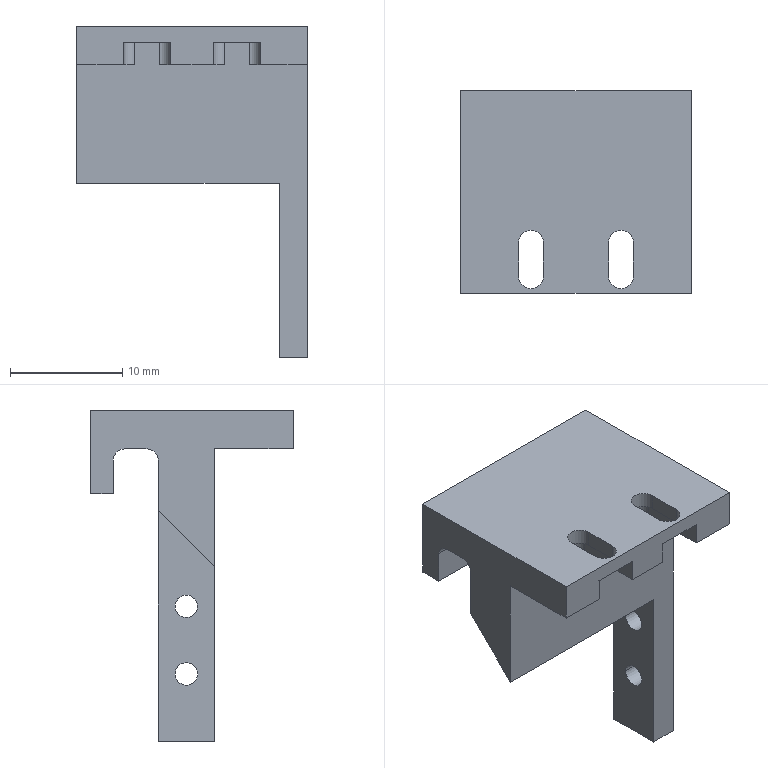Part | 1 solid | 42 faces | box 20.5 x 18 x 29.4 mm | volume 2312 mm3 | plane 26 | cylinder 16 | commonest cylinder face diameters 2 x10 2.2 x6
STEP:
#1=CARTESIAN_POINT('',(7.75,-0.5,-23.4));
#2=VERTEX_POINT('',#1);
#3=CARTESIAN_POINT('',(7.75,1.5,-23.4));
#4=VERTEX_POINT('',#3);
#5=CARTESIAN_POINT('',(7.75,0.5,-23.4));
#6=DIRECTION('',(-1.,0.,0.));
#7=DIRECTION('',(0.,1.,0.));
#8=AXIS2_PLACEMENT_3D('',#5,#6,#7);
#9=CIRCLE('',#8,1.);
#10=EDGE_CURVE('',#2,#4,#9,.T.);
#11=ORIENTED_EDGE('',*,*,#10,.T.);
#12=CARTESIAN_POINT('',(10.25,1.5,-23.4));
#13=VERTEX_POINT('',#12);
#14=CARTESIAN_POINT('',(10.25,1.5,-23.4));
#15=DIRECTION('',(1.,0.,0.));
#16=VECTOR('',#15,1000.);
#17=LINE('',#14,#16);
#18=EDGE_CURVE('',#13,#4,#17,.F.);
#19=ORIENTED_EDGE('',*,*,#18,.F.);
#20=CARTESIAN_POINT('',(10.25,-0.5,-23.4));
#21=VERTEX_POINT('',#20);
#22=CARTESIAN_POINT('',(10.25,0.5,-23.4));
#23=DIRECTION('',(1.,0.,0.));
#24=DIRECTION('',(0.,-1.,0.));
#25=AXIS2_PLACEMENT_3D('',#22,#23,#24);
#26=CIRCLE('',#25,1.);
#27=EDGE_CURVE('',#13,#21,#26,.T.);
#28=ORIENTED_EDGE('',*,*,#27,.T.);
#29=CARTESIAN_POINT('',(10.25,-0.5,-23.4));
#30=DIRECTION('',(1.,0.,0.));
#31=VECTOR('',#30,1000.);
#32=LINE('',#29,#31);
#33=EDGE_CURVE('',#21,#2,#32,.F.);
#34=ORIENTED_EDGE('',*,*,#33,.T.);
#35=EDGE_LOOP('',(#11,#19,#28,#34));
#36=FACE_BOUND('',#35,.T.);
#37=CARTESIAN_POINT('',(10.25,0.5,-23.4));
#38=DIRECTION('',(1.,0.,0.));
#39=DIRECTION('',(0.,1.,0.));
#40=AXIS2_PLACEMENT_3D('',#37,#38,#39);
#41=CYLINDRICAL_SURFACE('',#40,1.);
#42=ADVANCED_FACE('',(#36),#41,.F.);
#43=CARTESIAN_POINT('',(7.75,-0.5,-17.4));
#44=VERTEX_POINT('',#43);
#45=CARTESIAN_POINT('',(7.75,1.5,-17.4));
#46=VERTEX_POINT('',#45);
#47=CARTESIAN_POINT('',(7.75,0.5,-17.4));
#48=DIRECTION('',(-1.,0.,0.));
#49=DIRECTION('',(0.,1.,0.));
#50=AXIS2_PLACEMENT_3D('',#47,#48,#49);
#51=CIRCLE('',#50,1.);
#52=EDGE_CURVE('',#44,#46,#51,.T.);
#53=ORIENTED_EDGE('',*,*,#52,.T.);
#54=CARTESIAN_POINT('',(10.25,1.5,-17.4));
#55=VERTEX_POINT('',#54);
#56=CARTESIAN_POINT('',(10.25,1.5,-17.4));
#57=DIRECTION('',(1.,0.,0.));
#58=VECTOR('',#57,1000.);
#59=LINE('',#56,#58);
#60=EDGE_CURVE('',#55,#46,#59,.F.);
#61=ORIENTED_EDGE('',*,*,#60,.F.);
#62=CARTESIAN_POINT('',(10.25,-0.5,-17.4));
#63=VERTEX_POINT('',#62);
#64=CARTESIAN_POINT('',(10.25,0.5,-17.4));
#65=DIRECTION('',(1.,0.,0.));
#66=DIRECTION('',(0.,-1.,0.));
#67=AXIS2_PLACEMENT_3D('',#64,#65,#66);
#68=CIRCLE('',#67,1.);
#69=EDGE_CURVE('',#55,#63,#68,.T.);
#70=ORIENTED_EDGE('',*,*,#69,.T.);
#71=CARTESIAN_POINT('',(10.25,-0.5,-17.4));
#72=DIRECTION('',(1.,0.,0.));
#73=VECTOR('',#72,1000.);
#74=LINE('',#71,#73);
#75=EDGE_CURVE('',#63,#44,#74,.F.);
#76=ORIENTED_EDGE('',*,*,#75,.T.);
#77=EDGE_LOOP('',(#53,#61,#70,#76));
#78=FACE_BOUND('',#77,.T.);
#79=CARTESIAN_POINT('',(10.25,0.5,-17.4));
#80=DIRECTION('',(1.,0.,0.));
#81=DIRECTION('',(0.,1.,0.));
#82=AXIS2_PLACEMENT_3D('',#79,#80,#81);
#83=CYLINDRICAL_SURFACE('',#82,1.);
#84=ADVANCED_FACE('',(#78),#83,.F.);
#85=CARTESIAN_POINT('',(-4.,-8.6,0.));
#86=VERTEX_POINT('',#85);
#87=CARTESIAN_POINT('',(-5.1,-7.5,0.));
#88=VERTEX_POINT('',#87);
#89=CARTESIAN_POINT('',(-4.,-7.5,0.));
#90=DIRECTION('',(0.,0.,-1.));
#91=DIRECTION('',(0.,1.,0.));
#92=AXIS2_PLACEMENT_3D('',#89,#90,#91);
#93=CIRCLE('',#92,1.1);
#94=EDGE_CURVE('',#86,#88,#93,.T.);
#95=ORIENTED_EDGE('',*,*,#94,.F.);
#96=CARTESIAN_POINT('',(-4.,-8.6,-1.4));
#97=VERTEX_POINT('',#96);
#98=CARTESIAN_POINT('',(-4.,-8.6,0.));
#99=DIRECTION('',(0.,0.,-1.));
#100=VECTOR('',#99,1000.);
#101=LINE('',#98,#100);
#102=EDGE_CURVE('',#86,#97,#101,.T.);
#103=ORIENTED_EDGE('',*,*,#102,.T.);
#104=CARTESIAN_POINT('',(-5.1,-7.5,-1.4));
#105=VERTEX_POINT('',#104);
#106=CARTESIAN_POINT('',(-4.,-7.5,-1.4));
#107=DIRECTION('',(0.,0.,-1.));
#108=DIRECTION('',(0.,1.,0.));
#109=AXIS2_PLACEMENT_3D('',#106,#107,#108);
#110=CIRCLE('',#109,1.1);
#111=EDGE_CURVE('',#97,#105,#110,.T.);
#112=ORIENTED_EDGE('',*,*,#111,.T.);
#113=CARTESIAN_POINT('',(-5.1,-7.5,0.));
#114=DIRECTION('',(0.,0.,-1.));
#115=VECTOR('',#114,1000.);
#116=LINE('',#113,#115);
#117=EDGE_CURVE('',#88,#105,#116,.T.);
#118=ORIENTED_EDGE('',*,*,#117,.F.);
#119=EDGE_LOOP('',(#95,#103,#112,#118));
#120=FACE_BOUND('',#119,.T.);
#121=CARTESIAN_POINT('',(-4.,-7.5,0.));
#122=DIRECTION('',(0.,0.,-1.));
#123=DIRECTION('',(0.,1.,0.));
#124=AXIS2_PLACEMENT_3D('',#121,#122,#123);
#125=CYLINDRICAL_SURFACE('',#124,1.1);
#126=ADVANCED_FACE('',(#120),#125,.F.);
#127=CARTESIAN_POINT('',(4.,-8.6,0.));
#128=VERTEX_POINT('',#127);
#129=CARTESIAN_POINT('',(2.9,-7.5,0.));
#130=VERTEX_POINT('',#129);
#131=CARTESIAN_POINT('',(4.,-7.5,0.));
#132=DIRECTION('',(0.,0.,-1.));
#133=DIRECTION('',(0.,-1.,0.));
#134=AXIS2_PLACEMENT_3D('',#131,#132,#133);
#135=CIRCLE('',#134,1.1);
#136=EDGE_CURVE('',#128,#130,#135,.T.);
#137=ORIENTED_EDGE('',*,*,#136,.F.);
#138=CARTESIAN_POINT('',(4.,-8.6,-1.4));
#139=VERTEX_POINT('',#138);
#140=CARTESIAN_POINT('',(4.,-8.6,0.));
#141=DIRECTION('',(0.,0.,-1.));
#142=VECTOR('',#141,1000.);
#143=LINE('',#140,#142);
#144=EDGE_CURVE('',#128,#139,#143,.T.);
#145=ORIENTED_EDGE('',*,*,#144,.T.);
#146=CARTESIAN_POINT('',(2.9,-7.5,-1.4));
#147=VERTEX_POINT('',#146);
#148=CARTESIAN_POINT('',(4.,-7.5,-1.4));
#149=DIRECTION('',(0.,0.,1.));
#150=DIRECTION('',(0.,-1.,0.));
#151=AXIS2_PLACEMENT_3D('',#148,#149,#150);
#152=CIRCLE('',#151,1.1);
#153=EDGE_CURVE('',#147,#139,#152,.T.);
#154=ORIENTED_EDGE('',*,*,#153,.F.);
#155=CARTESIAN_POINT('',(2.9,-7.5,0.));
#156=DIRECTION('',(0.,0.,-1.));
#157=VECTOR('',#156,1000.);
#158=LINE('',#155,#157);
#159=EDGE_CURVE('',#130,#147,#158,.T.);
#160=ORIENTED_EDGE('',*,*,#159,.F.);
#161=EDGE_LOOP('',(#137,#145,#154,#160));
#162=FACE_BOUND('',#161,.T.);
#163=CARTESIAN_POINT('',(4.,-7.5,0.));
#164=DIRECTION('',(0.,0.,-1.));
#165=DIRECTION('',(0.,1.,0.));
#166=AXIS2_PLACEMENT_3D('',#163,#164,#165);
#167=CYLINDRICAL_SURFACE('',#166,1.1);
#168=ADVANCED_FACE('',(#162),#167,.F.);
#169=CARTESIAN_POINT('',(-2.9,-2.,-3.4));
#170=VERTEX_POINT('',#169);
#171=CARTESIAN_POINT('',(2.9,-2.,-3.4));
#172=VERTEX_POINT('',#171);
#173=CARTESIAN_POINT('',(-10.25,-2.,-3.4));
#174=DIRECTION('',(1.,0.,0.));
#175=VECTOR('',#174,1000.);
#176=LINE('',#173,#175);
#177=EDGE_CURVE('',#170,#172,#176,.T.);
#178=ORIENTED_EDGE('',*,*,#177,.T.);
#179=CARTESIAN_POINT('',(1.9,-3.,-3.4));
#180=VERTEX_POINT('',#179);
#181=CARTESIAN_POINT('',(2.9,-3.,-3.4));
#182=DIRECTION('',(0.,0.,1.));
#183=DIRECTION('',(0.,1.,0.));
#184=AXIS2_PLACEMENT_3D('',#181,#182,#183);
#185=CIRCLE('',#184,1.);
#186=EDGE_CURVE('',#172,#180,#185,.T.);
#187=ORIENTED_EDGE('',*,*,#186,.T.);
#188=CARTESIAN_POINT('',(1.9,-9.,-3.4));
#189=VERTEX_POINT('',#188);
#190=CARTESIAN_POINT('',(1.9,-9.,-3.4));
#191=DIRECTION('',(0.,1.,0.));
#192=VECTOR('',#191,1000.);
#193=LINE('',#190,#192);
#194=EDGE_CURVE('',#189,#180,#193,.T.);
#195=ORIENTED_EDGE('',*,*,#194,.F.);
#196=CARTESIAN_POINT('',(-1.9,-9.,-3.4));
#197=VERTEX_POINT('',#196);
#198=CARTESIAN_POINT('',(10.25,-9.,-3.4));
#199=DIRECTION('',(1.,0.,0.));
#200=VECTOR('',#199,1000.);
#201=LINE('',#198,#200);
#202=EDGE_CURVE('',#197,#189,#201,.T.);
#203=ORIENTED_EDGE('',*,*,#202,.F.);
#204=CARTESIAN_POINT('',(-1.9,-3.,-3.4));
#205=VERTEX_POINT('',#204);
#206=CARTESIAN_POINT('',(-1.9,-9.,-3.4));
#207=DIRECTION('',(0.,-1.,0.));
#208=VECTOR('',#207,1000.);
#209=LINE('',#206,#208);
#210=EDGE_CURVE('',#205,#197,#209,.T.);
#211=ORIENTED_EDGE('',*,*,#210,.F.);
#212=CARTESIAN_POINT('',(-2.9,-3.,-3.4));
#213=DIRECTION('',(0.,0.,1.));
#214=DIRECTION('',(0.,1.,0.));
#215=AXIS2_PLACEMENT_3D('',#212,#213,#214);
#216=CIRCLE('',#215,1.);
#217=EDGE_CURVE('',#205,#170,#216,.T.);
#218=ORIENTED_EDGE('',*,*,#217,.T.);
#219=EDGE_LOOP('',(#178,#187,#195,#203,#211,#218));
#220=FACE_BOUND('',#219,.T.);
#221=CARTESIAN_POINT('',(7.75,7.,-3.4));
#222=DIRECTION('',(0.,0.,1.));
#223=DIRECTION('',(0.,-1.,0.));
#224=AXIS2_PLACEMENT_3D('',#221,#222,#223);
#225=PLANE('',#224);
#226=ADVANCED_FACE('',(#220),#225,.F.);
#227=CARTESIAN_POINT('',(6.1,-9.,-3.4));
#228=VERTEX_POINT('',#227);
#229=CARTESIAN_POINT('',(10.25,-9.,-3.4));
#230=VERTEX_POINT('',#229);
#231=CARTESIAN_POINT('',(10.25,-9.,-3.4));
#232=DIRECTION('',(1.,0.,0.));
#233=VECTOR('',#232,1000.);
#234=LINE('',#231,#233);
#235=EDGE_CURVE('',#228,#230,#234,.T.);
#236=ORIENTED_EDGE('',*,*,#235,.F.);
#237=CARTESIAN_POINT('',(6.1,-3.,-3.4));
#238=VERTEX_POINT('',#237);
#239=CARTESIAN_POINT('',(6.1,-2.,-3.4));
#240=DIRECTION('',(0.,-1.,0.));
#241=VECTOR('',#240,1000.);
#242=LINE('',#239,#241);
#243=EDGE_CURVE('',#238,#228,#242,.T.);
#244=ORIENTED_EDGE('',*,*,#243,.F.);
#245=CARTESIAN_POINT('',(5.1,-2.,-3.4));
#246=VERTEX_POINT('',#245);
#247=CARTESIAN_POINT('',(5.1,-3.,-3.4));
#248=DIRECTION('',(0.,0.,1.));
#249=DIRECTION('',(0.,1.,0.));
#250=AXIS2_PLACEMENT_3D('',#247,#248,#249);
#251=CIRCLE('',#250,1.);
#252=EDGE_CURVE('',#238,#246,#251,.T.);
#253=ORIENTED_EDGE('',*,*,#252,.T.);
#254=CARTESIAN_POINT('',(10.25,-2.,-3.4));
#255=VERTEX_POINT('',#254);
#256=CARTESIAN_POINT('',(-10.25,-2.,-3.4));
#257=DIRECTION('',(1.,0.,0.));
#258=VECTOR('',#257,1000.);
#259=LINE('',#256,#258);
#260=EDGE_CURVE('',#246,#255,#259,.T.);
#261=ORIENTED_EDGE('',*,*,#260,.T.);
#262=CARTESIAN_POINT('',(10.25,-9.,-3.4));
#263=DIRECTION('',(0.,1.,0.));
#264=VECTOR('',#263,1000.);
#265=LINE('',#262,#264);
#266=EDGE_CURVE('',#230,#255,#265,.T.);
#267=ORIENTED_EDGE('',*,*,#266,.F.);
#268=EDGE_LOOP('',(#236,#244,#253,#261,#267));
#269=FACE_BOUND('',#268,.T.);
#270=CARTESIAN_POINT('',(7.75,7.,-3.4));
#271=DIRECTION('',(0.,0.,1.));
#272=DIRECTION('',(0.,-1.,0.));
#273=AXIS2_PLACEMENT_3D('',#270,#271,#272);
#274=PLANE('',#273);
#275=ADVANCED_FACE('',(#269),#274,.F.);
#276=ORIENTED_EDGE('',*,*,#144,.F.);
#277=CARTESIAN_POINT('',(5.1,-7.5,0.));
#278=VERTEX_POINT('',#277);
#279=CARTESIAN_POINT('',(4.,-7.5,0.));
#280=DIRECTION('',(0.,0.,-1.));
#281=DIRECTION('',(0.,-1.,0.));
#282=AXIS2_PLACEMENT_3D('',#279,#280,#281);
#283=CIRCLE('',#282,1.1);
#284=EDGE_CURVE('',#278,#128,#283,.T.);
#285=ORIENTED_EDGE('',*,*,#284,.F.);
#286=CARTESIAN_POINT('',(5.1,-7.5,-1.4));
#287=VERTEX_POINT('',#286);
#288=CARTESIAN_POINT('',(5.1,-7.5,0.));
#289=DIRECTION('',(0.,0.,-1.));
#290=VECTOR('',#289,1000.);
#291=LINE('',#288,#290);
#292=EDGE_CURVE('',#278,#287,#291,.T.);
#293=ORIENTED_EDGE('',*,*,#292,.T.);
#294=CARTESIAN_POINT('',(4.,-7.5,-1.4));
#295=DIRECTION('',(0.,0.,1.));
#296=DIRECTION('',(0.,-1.,0.));
#297=AXIS2_PLACEMENT_3D('',#294,#295,#296);
#298=CIRCLE('',#297,1.1);
#299=EDGE_CURVE('',#139,#287,#298,.T.);
#300=ORIENTED_EDGE('',*,*,#299,.F.);
#301=EDGE_LOOP('',(#276,#285,#293,#300));
#302=FACE_BOUND('',#301,.T.);
#303=CARTESIAN_POINT('',(4.,-7.5,0.));
#304=DIRECTION('',(0.,0.,-1.));
#305=DIRECTION('',(0.,1.,0.));
#306=AXIS2_PLACEMENT_3D('',#303,#304,#305);
#307=CYLINDRICAL_SURFACE('',#306,1.1);
#308=ADVANCED_FACE('',(#302),#307,.F.);
#309=CARTESIAN_POINT('',(5.1,-4.5,-1.4));
#310=VERTEX_POINT('',#309);
#311=CARTESIAN_POINT('',(5.1,-7.5,-1.4));
#312=DIRECTION('',(0.,1.,0.));
#313=VECTOR('',#312,1000.);
#314=LINE('',#311,#313);
#315=EDGE_CURVE('',#287,#310,#314,.T.);
#316=ORIENTED_EDGE('',*,*,#315,.F.);
#317=ORIENTED_EDGE('',*,*,#292,.F.);
#318=CARTESIAN_POINT('',(5.1,-4.5,0.));
#319=VERTEX_POINT('',#318);
#320=CARTESIAN_POINT('',(5.1,-7.5,0.));
#321=DIRECTION('',(0.,-1.,0.));
#322=VECTOR('',#321,1000.);
#323=LINE('',#320,#322);
#324=EDGE_CURVE('',#319,#278,#323,.T.);
#325=ORIENTED_EDGE('',*,*,#324,.F.);
#326=CARTESIAN_POINT('',(5.1,-4.5,0.));
#327=DIRECTION('',(0.,0.,-1.));
#328=VECTOR('',#327,1000.);
#329=LINE('',#326,#328);
#330=EDGE_CURVE('',#319,#310,#329,.T.);
#331=ORIENTED_EDGE('',*,*,#330,.T.);
#332=EDGE_LOOP('',(#316,#317,#325,#331));
#333=FACE_BOUND('',#332,.T.);
#334=CARTESIAN_POINT('',(5.1,-7.5,0.));
#335=DIRECTION('',(1.,0.,0.));
#336=DIRECTION('',(0.,1.,0.));
#337=AXIS2_PLACEMENT_3D('',#334,#335,#336);
#338=PLANE('',#337);
#339=ADVANCED_FACE('',(#333),#338,.F.);
#340=CARTESIAN_POINT('',(2.9,-4.5,-1.4));
#341=VERTEX_POINT('',#340);
#342=CARTESIAN_POINT('',(4.,-4.5,-1.4));
#343=DIRECTION('',(0.,0.,1.));
#344=DIRECTION('',(0.,-1.,0.));
#345=AXIS2_PLACEMENT_3D('',#342,#343,#344);
#346=CIRCLE('',#345,1.1);
#347=EDGE_CURVE('',#310,#341,#346,.T.);
#348=ORIENTED_EDGE('',*,*,#347,.F.);
#349=ORIENTED_EDGE('',*,*,#330,.F.);
#350=CARTESIAN_POINT('',(2.9,-4.5,0.));
#351=VERTEX_POINT('',#350);
#352=CARTESIAN_POINT('',(4.,-4.5,0.));
#353=DIRECTION('',(0.,0.,-1.));
#354=DIRECTION('',(0.,-1.,0.));
#355=AXIS2_PLACEMENT_3D('',#352,#353,#354);
#356=CIRCLE('',#355,1.1);
#357=EDGE_CURVE('',#351,#319,#356,.T.);
#358=ORIENTED_EDGE('',*,*,#357,.F.);
#359=CARTESIAN_POINT('',(2.9,-4.5,0.));
#360=DIRECTION('',(0.,0.,-1.));
#361=VECTOR('',#360,1000.);
#362=LINE('',#359,#361);
#363=EDGE_CURVE('',#351,#341,#362,.T.);
#364=ORIENTED_EDGE('',*,*,#363,.T.);
#365=EDGE_LOOP('',(#348,#349,#358,#364));
#366=FACE_BOUND('',#365,.T.);
#367=CARTESIAN_POINT('',(4.,-4.5,0.));
#368=DIRECTION('',(0.,0.,-1.));
#369=DIRECTION('',(0.,1.,0.));
#370=AXIS2_PLACEMENT_3D('',#367,#368,#369);
#371=CYLINDRICAL_SURFACE('',#370,1.1);
#372=ADVANCED_FACE('',(#366),#371,.F.);
#373=CARTESIAN_POINT('',(2.9,-7.5,-1.4));
#374=DIRECTION('',(0.,-1.,0.));
#375=VECTOR('',#374,1000.);
#376=LINE('',#373,#375);
#377=EDGE_CURVE('',#341,#147,#376,.T.);
#378=ORIENTED_EDGE('',*,*,#377,.F.);
#379=ORIENTED_EDGE('',*,*,#363,.F.);
#380=CARTESIAN_POINT('',(2.9,-7.5,0.));
#381=DIRECTION('',(0.,1.,0.));
#382=VECTOR('',#381,1000.);
#383=LINE('',#380,#382);
#384=EDGE_CURVE('',#130,#351,#383,.T.);
#385=ORIENTED_EDGE('',*,*,#384,.F.);
#386=ORIENTED_EDGE('',*,*,#159,.T.);
#387=EDGE_LOOP('',(#378,#379,#385,#386));
#388=FACE_BOUND('',#387,.T.);
#389=CARTESIAN_POINT('',(2.9,-7.5,0.));
#390=DIRECTION('',(-1.,0.,0.));
#391=DIRECTION('',(0.,-1.,0.));
#392=AXIS2_PLACEMENT_3D('',#389,#390,#391);
#393=PLANE('',#392);
#394=ADVANCED_FACE('',(#388),#393,.F.);
#395=CARTESIAN_POINT('',(10.25,4.,-3.4));
#396=VERTEX_POINT('',#395);
#397=CARTESIAN_POINT('',(10.25,6.,-3.4));
#398=VERTEX_POINT('',#397);
#399=CARTESIAN_POINT('',(10.25,-9.,-3.4));
#400=DIRECTION('',(0.,1.,0.));
#401=VECTOR('',#400,1000.);
#402=LINE('',#399,#401);
#403=EDGE_CURVE('',#396,#398,#402,.T.);
#404=ORIENTED_EDGE('',*,*,#403,.F.);
#405=CARTESIAN_POINT('',(-10.25,4.,-3.4));
#406=VERTEX_POINT('',#405);
#407=CARTESIAN_POINT('',(-10.25,4.,-3.4));
#408=DIRECTION('',(-1.,0.,0.));
#409=VECTOR('',#408,1000.);
#410=LINE('',#407,#409);
#411=EDGE_CURVE('',#396,#406,#410,.T.);
#412=ORIENTED_EDGE('',*,*,#411,.T.);
#413=CARTESIAN_POINT('',(-10.25,6.,-3.4));
#414=VERTEX_POINT('',#413);
#415=CARTESIAN_POINT('',(-10.25,9.,-3.4));
#416=DIRECTION('',(0.,-1.,0.));
#417=VECTOR('',#416,1000.);
#418=LINE('',#415,#417);
#419=EDGE_CURVE('',#414,#406,#418,.T.);
#420=ORIENTED_EDGE('',*,*,#419,.F.);
#421=CARTESIAN_POINT('',(10.25,6.,-3.4));
#422=DIRECTION('',(1.,0.,0.));
#423=VECTOR('',#422,1000.);
#424=LINE('',#421,#423);
#425=EDGE_CURVE('',#414,#398,#424,.T.);
#426=ORIENTED_EDGE('',*,*,#425,.T.);
#427=EDGE_LOOP('',(#404,#412,#420,#426));
#428=FACE_BOUND('',#427,.T.);
#429=CARTESIAN_POINT('',(7.75,7.,-3.4));
#430=DIRECTION('',(0.,0.,1.));
#431=DIRECTION('',(0.,-1.,0.));
#432=AXIS2_PLACEMENT_3D('',#429,#430,#431);
#433=PLANE('',#432);
#434=ADVANCED_FACE('',(#428),#433,.F.);
#435=CARTESIAN_POINT('',(-5.1,-2.,-1.4));
#436=VERTEX_POINT('',#435);
#437=CARTESIAN_POINT('',(-2.9,-2.,-1.4));
#438=VERTEX_POINT('',#437);
#439=CARTESIAN_POINT('',(-1.9,-2.,-1.4));
#440=DIRECTION('',(1.,0.,0.));
#441=VECTOR('',#440,1000.);
#442=LINE('',#439,#441);
#443=EDGE_CURVE('',#436,#438,#442,.T.);
#444=ORIENTED_EDGE('',*,*,#443,.F.);
#445=CARTESIAN_POINT('',(-5.1,-2.,-3.4));
#446=VERTEX_POINT('',#445);
#447=CARTESIAN_POINT('',(-5.1,-2.,-3.4));
#448=DIRECTION('',(0.,0.,-1.));
#449=VECTOR('',#448,1000.);
#450=LINE('',#447,#449);
#451=EDGE_CURVE('',#436,#446,#450,.T.);
#452=ORIENTED_EDGE('',*,*,#451,.T.);
#453=CARTESIAN_POINT('',(-10.25,-2.,-3.4));
#454=VERTEX_POINT('',#453);
#455=CARTESIAN_POINT('',(-10.25,-2.,-3.4));
#456=DIRECTION('',(1.,0.,0.));
#457=VECTOR('',#456,1000.);
#458=LINE('',#455,#457);
#459=EDGE_CURVE('',#454,#446,#458,.T.);
#460=ORIENTED_EDGE('',*,*,#459,.F.);
#461=CARTESIAN_POINT('',(-10.25,-2.,-13.9));
#462=VERTEX_POINT('',#461);
#463=CARTESIAN_POINT('',(-10.25,-2.,-3.4));
#464=DIRECTION('',(0.,0.,1.));
#465=VECTOR('',#464,1000.);
#466=LINE('',#463,#465);
#467=EDGE_CURVE('',#462,#454,#466,.T.);
#468=ORIENTED_EDGE('',*,*,#467,.F.);
#469=CARTESIAN_POINT('',(7.75,-2.,-13.9));
#470=VERTEX_POINT('',#469);
#471=CARTESIAN_POINT('',(-10.25,-2.,-13.9));
#472=DIRECTION('',(1.,0.,0.));
#473=VECTOR('',#472,1000.);
#474=LINE('',#471,#473);
#475=EDGE_CURVE('',#462,#470,#474,.T.);
#476=ORIENTED_EDGE('',*,*,#475,.T.);
#477=CARTESIAN_POINT('',(7.75,-2.,-29.4));
#478=VERTEX_POINT('',#477);
#479=CARTESIAN_POINT('',(7.75,-2.,-29.4));
#480=DIRECTION('',(0.,0.,1.));
#481=VECTOR('',#480,1000.);
#482=LINE('',#479,#481);
#483=EDGE_CURVE('',#478,#470,#482,.T.);
#484=ORIENTED_EDGE('',*,*,#483,.F.);
#485=CARTESIAN_POINT('',(10.25,-2.,-29.4));
#486=VERTEX_POINT('',#485);
#487=CARTESIAN_POINT('',(7.75,-2.,-29.4));
#488=DIRECTION('',(1.,0.,0.));
#489=VECTOR('',#488,1000.);
#490=LINE('',#487,#489);
#491=EDGE_CURVE('',#478,#486,#490,.T.);
#492=ORIENTED_EDGE('',*,*,#491,.T.);
#493=CARTESIAN_POINT('',(10.25,-2.,-29.4));
#494=DIRECTION('',(0.,0.,1.));
#495=VECTOR('',#494,1000.);
#496=LINE('',#493,#495);
#497=EDGE_CURVE('',#486,#255,#496,.T.);
#498=ORIENTED_EDGE('',*,*,#497,.T.);
#499=ORIENTED_EDGE('',*,*,#260,.F.);
#500=CARTESIAN_POINT('',(5.1,-2.,-1.4));
#501=VERTEX_POINT('',#500);
#502=CARTESIAN_POINT('',(5.1,-2.,-1.4));
#503=DIRECTION('',(0.,0.,1.));
#504=VECTOR('',#503,1000.);
#505=LINE('',#502,#504);
#506=EDGE_CURVE('',#246,#501,#505,.T.);
#507=ORIENTED_EDGE('',*,*,#506,.T.);
#508=CARTESIAN_POINT('',(2.9,-2.,-1.4));
#509=VERTEX_POINT('',#508);
#510=CARTESIAN_POINT('',(1.9,-2.,-1.4));
#511=DIRECTION('',(1.,0.,0.));
#512=VECTOR('',#511,1000.);
#513=LINE('',#510,#512);
#514=EDGE_CURVE('',#509,#501,#513,.T.);
#515=ORIENTED_EDGE('',*,*,#514,.F.);
#516=CARTESIAN_POINT('',(2.9,-2.,-3.4));
#517=DIRECTION('',(0.,0.,-1.));
#518=VECTOR('',#517,1000.);
#519=LINE('',#516,#518);
#520=EDGE_CURVE('',#509,#172,#519,.T.);
#521=ORIENTED_EDGE('',*,*,#520,.T.);
#522=ORIENTED_EDGE('',*,*,#177,.F.);
#523=CARTESIAN_POINT('',(-2.9,-2.,-1.4));
#524=DIRECTION('',(0.,0.,1.));
#525=VECTOR('',#524,1000.);
#526=LINE('',#523,#525);
#527=EDGE_CURVE('',#170,#438,#526,.T.);
#528=ORIENTED_EDGE('',*,*,#527,.T.);
#529=EDGE_LOOP('',(#444,#452,#460,#468,#476,#484,#492,#498,#499,#507,#515,#521,#522,#528));
#530=FACE_BOUND('',#529,.T.);
#531=CARTESIAN_POINT('',(-10.25,-2.,-3.4));
#532=DIRECTION('',(0.,1.,0.));
#533=DIRECTION('',(-1.,0.,0.));
#534=AXIS2_PLACEMENT_3D('',#531,#532,#533);
#535=PLANE('',#534);
#536=ADVANCED_FACE('',(#530),#535,.F.);
#537=CARTESIAN_POINT('',(-10.25,3.,-4.4));
#538=VERTEX_POINT('',#537);
#539=CARTESIAN_POINT('',(-10.25,3.,-8.9));
#540=VERTEX_POINT('',#539);
#541=CARTESIAN_POINT('',(-10.25,3.,-8.9));
#542=DIRECTION('',(0.,0.,-1.));
#543=VECTOR('',#542,1000.);
#544=LINE('',#541,#543);
#545=EDGE_CURVE('',#538,#540,#544,.T.);
#546=ORIENTED_EDGE('',*,*,#545,.F.);
#547=CARTESIAN_POINT('',(10.25,3.,-4.4));
#548=VERTEX_POINT('',#547);
#549=CARTESIAN_POINT('',(10.25,3.,-4.4));
#550=DIRECTION('',(1.,0.,0.));
#551=VECTOR('',#550,1000.);
#552=LINE('',#549,#551);
#553=EDGE_CURVE('',#538,#548,#552,.T.);
#554=ORIENTED_EDGE('',*,*,#553,.T.);
#555=CARTESIAN_POINT('',(10.25,3.,-29.4));
#556=VERTEX_POINT('',#555);
#557=CARTESIAN_POINT('',(10.25,3.,-29.4));
#558=DIRECTION('',(0.,0.,1.));
#559=VECTOR('',#558,1000.);
#560=LINE('',#557,#559);
#561=EDGE_CURVE('',#556,#548,#560,.T.);
#562=ORIENTED_EDGE('',*,*,#561,.F.);
#563=CARTESIAN_POINT('',(7.75,3.,-29.4));
#564=VERTEX_POINT('',#563);
#565=CARTESIAN_POINT('',(10.25,3.,-29.4));
#566=DIRECTION('',(-1.,0.,0.));
#567=VECTOR('',#566,1000.);
#568=LINE('',#565,#567);
#569=EDGE_CURVE('',#556,#564,#568,.T.);
#570=ORIENTED_EDGE('',*,*,#569,.T.);
#571=CARTESIAN_POINT('',(7.75,3.,-8.9));
#572=VERTEX_POINT('',#571);
#573=CARTESIAN_POINT('',(7.75,3.,-29.4));
#574=DIRECTION('',(0.,0.,1.));
#575=VECTOR('',#574,1000.);
#576=LINE('',#573,#575);
#577=EDGE_CURVE('',#564,#572,#576,.T.);
#578=ORIENTED_EDGE('',*,*,#577,.T.);
#579=CARTESIAN_POINT('',(-10.25,3.,-8.9));
#580=DIRECTION('',(1.,0.,0.));
#581=VECTOR('',#580,1000.);
#582=LINE('',#579,#581);
#583=EDGE_CURVE('',#540,#572,#582,.T.);
#584=ORIENTED_EDGE('',*,*,#583,.F.);
#585=EDGE_LOOP('',(#546,#554,#562,#570,#578,#584));
#586=FACE_BOUND('',#585,.T.);
#587=CARTESIAN_POINT('',(-10.25,3.,-8.9));
#588=DIRECTION('',(0.,-1.,0.));
#589=DIRECTION('',(0.,0.,-1.));
#590=AXIS2_PLACEMENT_3D('',#587,#588,#589);
#591=PLANE('',#590);
#592=ADVANCED_FACE('',(#586),#591,.F.);
#593=CARTESIAN_POINT('',(7.75,-2.,-13.9));
#594=DIRECTION('',(0.,-0.7071,-0.7071));
#595=VECTOR('',#594,1000.);
#596=LINE('',#593,#595);
#597=EDGE_CURVE('',#572,#470,#596,.T.);
#598=ORIENTED_EDGE('',*,*,#597,.T.);
#599=ORIENTED_EDGE('',*,*,#475,.F.);
#600=CARTESIAN_POINT('',(-10.25,-2.,-13.9));
#601=DIRECTION('',(0.,-0.7071,-0.7071));
#602=VECTOR('',#601,1000.);
#603=LINE('',#600,#602);
#604=EDGE_CURVE('',#540,#462,#603,.T.);
#605=ORIENTED_EDGE('',*,*,#604,.F.);
#606=ORIENTED_EDGE('',*,*,#583,.T.);
#607=EDGE_LOOP('',(#598,#599,#605,#606));
#608=FACE_BOUND('',#607,.T.);
#609=CARTESIAN_POINT('',(-10.25,-2.,-13.9));
#610=DIRECTION('',(0.,-0.7071,0.7071));
#611=DIRECTION('',(0.,-0.7071,-0.7071));
#612=AXIS2_PLACEMENT_3D('',#609,#610,#611);
#613=PLANE('',#612);
#614=ADVANCED_FACE('',(#608),#613,.F.);
#615=ORIENTED_EDGE('',*,*,#467,.T.);
#616=CARTESIAN_POINT('',(-10.25,-9.,-3.4));
#617=VERTEX_POINT('',#616);
#618=CARTESIAN_POINT('',(-10.25,9.,-3.4));
#619=DIRECTION('',(0.,-1.,0.));
#620=VECTOR('',#619,1000.);
#621=LINE('',#618,#620);
#622=EDGE_CURVE('',#454,#617,#621,.T.);
#623=ORIENTED_EDGE('',*,*,#622,.T.);
#624=CARTESIAN_POINT('',(-10.25,-9.,0.));
#625=VERTEX_POINT('',#624);
#626=CARTESIAN_POINT('',(-10.25,-9.,0.));
#627=DIRECTION('',(0.,0.,-1.));
#628=VECTOR('',#627,1000.);
#629=LINE('',#626,#628);
#630=EDGE_CURVE('',#625,#617,#629,.T.);
#631=ORIENTED_EDGE('',*,*,#630,.F.);
#632=CARTESIAN_POINT('',(-10.25,9.,0.));
#633=VERTEX_POINT('',#632);
#634=CARTESIAN_POINT('',(-10.25,9.,0.));
#635=DIRECTION('',(0.,-1.,0.));
#636=VECTOR('',#635,1000.);
#637=LINE('',#634,#636);
#638=EDGE_CURVE('',#633,#625,#637,.T.);
#639=ORIENTED_EDGE('',*,*,#638,.F.);
#640=CARTESIAN_POINT('',(-10.25,9.,-7.4));
#641=VERTEX_POINT('',#640);
#642=CARTESIAN_POINT('',(-10.25,9.,0.));
#643=DIRECTION('',(0.,0.,-1.));
#644=VECTOR('',#643,1000.);
#645=LINE('',#642,#644);
#646=EDGE_CURVE('',#633,#641,#645,.T.);
#647=ORIENTED_EDGE('',*,*,#646,.T.);
#648=CARTESIAN_POINT('',(-10.25,7.,-7.4));
#649=VERTEX_POINT('',#648);
#650=CARTESIAN_POINT('',(-10.25,7.,-7.4));
#651=DIRECTION('',(0.,1.,0.));
#652=VECTOR('',#651,1000.);
#653=LINE('',#650,#652);
#654=EDGE_CURVE('',#649,#641,#653,.T.);
#655=ORIENTED_EDGE('',*,*,#654,.F.);
#656=CARTESIAN_POINT('',(-10.25,7.,-4.4));
#657=VERTEX_POINT('',#656);
#658=CARTESIAN_POINT('',(-10.25,7.,-7.4));
#659=DIRECTION('',(0.,0.,1.));
#660=VECTOR('',#659,1000.);
#661=LINE('',#658,#660);
#662=EDGE_CURVE('',#649,#657,#661,.T.);
#663=ORIENTED_EDGE('',*,*,#662,.T.);
#664=CARTESIAN_POINT('',(-10.25,6.,-4.4));
#665=DIRECTION('',(1.,0.,0.));
#666=DIRECTION('',(0.,1.,0.));
#667=AXIS2_PLACEMENT_3D('',#664,#665,#666);
#668=CIRCLE('',#667,1.);
#669=EDGE_CURVE('',#657,#414,#668,.T.);
#670=ORIENTED_EDGE('',*,*,#669,.T.);
#671=ORIENTED_EDGE('',*,*,#419,.T.);
#672=CARTESIAN_POINT('',(-10.25,4.,-4.4));
#673=DIRECTION('',(1.,0.,0.));
#674=DIRECTION('',(0.,1.,0.));
#675=AXIS2_PLACEMENT_3D('',#672,#673,#674);
#676=CIRCLE('',#675,1.);
#677=EDGE_CURVE('',#406,#538,#676,.T.);
#678=ORIENTED_EDGE('',*,*,#677,.T.);
#679=ORIENTED_EDGE('',*,*,#545,.T.);
#680=ORIENTED_EDGE('',*,*,#604,.T.);
#681=EDGE_LOOP('',(#615,#623,#631,#639,#647,#655,#663,#670,#671,#678,#679,#680));
#682=FACE_BOUND('',#681,.T.);
#683=CARTESIAN_POINT('',(-10.25,7.,-15.507));
#684=DIRECTION('',(-1.,0.,0.));
#685=DIRECTION('',(0.,-1.,0.));
#686=AXIS2_PLACEMENT_3D('',#683,#684,#685);
#687=PLANE('',#686);
#688=ADVANCED_FACE('',(#682),#687,.T.);
#689=ORIENTED_EDGE('',*,*,#10,.F.);
#690=CARTESIAN_POINT('',(7.75,0.5,-23.4));
#691=DIRECTION('',(-1.,0.,0.));
#692=DIRECTION('',(0.,1.,0.));
#693=AXIS2_PLACEMENT_3D('',#690,#691,#692);
#694=CIRCLE('',#693,1.);
#695=EDGE_CURVE('',#4,#2,#694,.T.);
#696=ORIENTED_EDGE('',*,*,#695,.F.);
#697=EDGE_LOOP('',(#689,#696));
#698=FACE_BOUND('',#697,.T.);
#699=ORIENTED_EDGE('',*,*,#52,.F.);
#700=CARTESIAN_POINT('',(7.75,0.5,-17.4));
#701=DIRECTION('',(-1.,0.,0.));
#702=DIRECTION('',(0.,1.,0.));
#703=AXIS2_PLACEMENT_3D('',#700,#701,#702);
#704=CIRCLE('',#703,1.);
#705=EDGE_CURVE('',#46,#44,#704,.T.);
#706=ORIENTED_EDGE('',*,*,#705,.F.);
#707=EDGE_LOOP('',(#699,#706));
#708=FACE_BOUND('',#707,.T.);
#709=ORIENTED_EDGE('',*,*,#597,.F.);
#710=ORIENTED_EDGE('',*,*,#577,.F.);
#711=CARTESIAN_POINT('',(7.75,3.,-29.4));
#712=DIRECTION('',(0.,-1.,0.));
#713=VECTOR('',#712,1000.);
#714=LINE('',#711,#713);
#715=EDGE_CURVE('',#564,#478,#714,.T.);
#716=ORIENTED_EDGE('',*,*,#715,.T.);
#717=ORIENTED_EDGE('',*,*,#483,.T.);
#718=EDGE_LOOP('',(#709,#710,#716,#717));
#719=FACE_BOUND('',#718,.T.);
#720=CARTESIAN_POINT('',(7.75,3.,-29.4));
#721=DIRECTION('',(-1.,0.,0.));
#722=DIRECTION('',(0.,-1.,0.));
#723=AXIS2_PLACEMENT_3D('',#720,#721,#722);
#724=PLANE('',#723);
#725=ADVANCED_FACE('',(#698,#708,#719),#724,.T.);
#726=CARTESIAN_POINT('',(10.25,0.5,-23.4));
#727=DIRECTION('',(1.,0.,0.));
#728=DIRECTION('',(0.,-1.,0.));
#729=AXIS2_PLACEMENT_3D('',#726,#727,#728);
#730=CIRCLE('',#729,1.);
#731=EDGE_CURVE('',#21,#13,#730,.T.);
#732=ORIENTED_EDGE('',*,*,#731,.F.);
#733=ORIENTED_EDGE('',*,*,#27,.F.);
#734=EDGE_LOOP('',(#732,#733));
#735=FACE_BOUND('',#734,.T.);
#736=CARTESIAN_POINT('',(10.25,0.5,-17.4));
#737=DIRECTION('',(1.,0.,0.));
#738=DIRECTION('',(0.,-1.,0.));
#739=AXIS2_PLACEMENT_3D('',#736,#737,#738);
#740=CIRCLE('',#739,1.);
#741=EDGE_CURVE('',#63,#55,#740,.T.);
#742=ORIENTED_EDGE('',*,*,#741,.F.);
#743=ORIENTED_EDGE('',*,*,#69,.F.);
#744=EDGE_LOOP('',(#742,#743));
#745=FACE_BOUND('',#744,.T.);
#746=ORIENTED_EDGE('',*,*,#561,.T.);
#747=CARTESIAN_POINT('',(10.25,4.,-4.4));
#748=DIRECTION('',(-1.,0.,0.));
#749=DIRECTION('',(0.,-1.,0.));
#750=AXIS2_PLACEMENT_3D('',#747,#748,#749);
#751=CIRCLE('',#750,1.);
#752=EDGE_CURVE('',#548,#396,#751,.T.);
#753=ORIENTED_EDGE('',*,*,#752,.T.);
#754=ORIENTED_EDGE('',*,*,#403,.T.);
#755=CARTESIAN_POINT('',(10.25,7.,-4.4));
#756=VERTEX_POINT('',#755);
#757=CARTESIAN_POINT('',(10.25,6.,-4.4));
#758=DIRECTION('',(-1.,0.,0.));
#759=DIRECTION('',(0.,-1.,0.));
#760=AXIS2_PLACEMENT_3D('',#757,#758,#759);
#761=CIRCLE('',#760,1.);
#762=EDGE_CURVE('',#398,#756,#761,.T.);
#763=ORIENTED_EDGE('',*,*,#762,.T.);
#764=CARTESIAN_POINT('',(10.25,7.,-7.4));
#765=VERTEX_POINT('',#764);
#766=CARTESIAN_POINT('',(10.25,7.,-7.4));
#767=DIRECTION('',(0.,0.,1.));
#768=VECTOR('',#767,1000.);
#769=LINE('',#766,#768);
#770=EDGE_CURVE('',#765,#756,#769,.T.);
#771=ORIENTED_EDGE('',*,*,#770,.F.);
#772=CARTESIAN_POINT('',(10.25,9.,-7.4));
#773=VERTEX_POINT('',#772);
#774=CARTESIAN_POINT('',(10.25,9.,-7.4));
#775=DIRECTION('',(0.,-1.,0.));
#776=VECTOR('',#775,1000.);
#777=LINE('',#774,#776);
#778=EDGE_CURVE('',#773,#765,#777,.T.);
#779=ORIENTED_EDGE('',*,*,#778,.F.);
#780=CARTESIAN_POINT('',(10.25,9.,0.));
#781=VERTEX_POINT('',#780);
#782=CARTESIAN_POINT('',(10.25,9.,0.));
#783=DIRECTION('',(0.,0.,-1.));
#784=VECTOR('',#783,1000.);
#785=LINE('',#782,#784);
#786=EDGE_CURVE('',#781,#773,#785,.T.);
#787=ORIENTED_EDGE('',*,*,#786,.F.);
#788=CARTESIAN_POINT('',(10.25,-9.,0.));
#789=VERTEX_POINT('',#788);
#790=CARTESIAN_POINT('',(10.25,-9.,0.));
#791=DIRECTION('',(0.,1.,0.));
#792=VECTOR('',#791,1000.);
#793=LINE('',#790,#792);
#794=EDGE_CURVE('',#789,#781,#793,.T.);
#795=ORIENTED_EDGE('',*,*,#794,.F.);
#796=CARTESIAN_POINT('',(10.25,-9.,0.));
#797=DIRECTION('',(0.,0.,-1.));
#798=VECTOR('',#797,1000.);
#799=LINE('',#796,#798);
#800=EDGE_CURVE('',#789,#230,#799,.T.);
#801=ORIENTED_EDGE('',*,*,#800,.T.);
#802=ORIENTED_EDGE('',*,*,#266,.T.);
#803=ORIENTED_EDGE('',*,*,#497,.F.);
#804=CARTESIAN_POINT('',(10.25,-2.,-29.4));
#805=DIRECTION('',(0.,1.,0.));
#806=VECTOR('',#805,1000.);
#807=LINE('',#804,#806);
#808=EDGE_CURVE('',#486,#556,#807,.T.);
#809=ORIENTED_EDGE('',*,*,#808,.T.);
#810=EDGE_LOOP('',(#746,#753,#754,#763,#771,#779,#787,#795,#801,#802,#803,#809));
#811=FACE_BOUND('',#810,.T.);
#812=CARTESIAN_POINT('',(10.25,-2.,-29.4));
#813=DIRECTION('',(1.,0.,0.));
#814=DIRECTION('',(0.,1.,0.));
#815=AXIS2_PLACEMENT_3D('',#812,#813,#814);
#816=PLANE('',#815);
#817=ADVANCED_FACE('',(#735,#745,#811),#816,.T.);
#818=ORIENTED_EDGE('',*,*,#715,.F.);
#819=ORIENTED_EDGE('',*,*,#569,.F.);
#820=ORIENTED_EDGE('',*,*,#808,.F.);
#821=ORIENTED_EDGE('',*,*,#491,.F.);
#822=EDGE_LOOP('',(#818,#819,#820,#821));
#823=FACE_BOUND('',#822,.T.);
#824=CARTESIAN_POINT('',(7.75,7.,-29.4));
#825=DIRECTION('',(0.,0.,1.));
#826=DIRECTION('',(0.,-1.,0.));
#827=AXIS2_PLACEMENT_3D('',#824,#825,#826);
#828=PLANE('',#827);
#829=ADVANCED_FACE('',(#823),#828,.F.);
#830=ORIENTED_EDGE('',*,*,#459,.T.);
#831=CARTESIAN_POINT('',(-6.1,-3.,-3.4));
#832=VERTEX_POINT('',#831);
#833=CARTESIAN_POINT('',(-5.1,-3.,-3.4));
#834=DIRECTION('',(0.,0.,1.));
#835=DIRECTION('',(0.,1.,0.));
#836=AXIS2_PLACEMENT_3D('',#833,#834,#835);
#837=CIRCLE('',#836,1.);
#838=EDGE_CURVE('',#446,#832,#837,.T.);
#839=ORIENTED_EDGE('',*,*,#838,.T.);
#840=CARTESIAN_POINT('',(-6.1,-9.,-3.4));
#841=VERTEX_POINT('',#840);
#842=CARTESIAN_POINT('',(-6.1,-2.,-3.4));
#843=DIRECTION('',(0.,1.,0.));
#844=VECTOR('',#843,1000.);
#845=LINE('',#842,#844);
#846=EDGE_CURVE('',#841,#832,#845,.T.);
#847=ORIENTED_EDGE('',*,*,#846,.F.);
#848=CARTESIAN_POINT('',(10.25,-9.,-3.4));
#849=DIRECTION('',(1.,0.,0.));
#850=VECTOR('',#849,1000.);
#851=LINE('',#848,#850);
#852=EDGE_CURVE('',#617,#841,#851,.T.);
#853=ORIENTED_EDGE('',*,*,#852,.F.);
#854=ORIENTED_EDGE('',*,*,#622,.F.);
#855=EDGE_LOOP('',(#830,#839,#847,#853,#854));
#856=FACE_BOUND('',#855,.T.);
#857=CARTESIAN_POINT('',(7.75,7.,-3.4));
#858=DIRECTION('',(0.,0.,1.));
#859=DIRECTION('',(0.,-1.,0.));
#860=AXIS2_PLACEMENT_3D('',#857,#858,#859);
#861=PLANE('',#860);
#862=ADVANCED_FACE('',(#856),#861,.F.);
#863=ORIENTED_EDGE('',*,*,#786,.T.);
#864=CARTESIAN_POINT('',(10.25,9.,-7.4));
#865=DIRECTION('',(1.,0.,0.));
#866=VECTOR('',#865,1000.);
#867=LINE('',#864,#866);
#868=EDGE_CURVE('',#641,#773,#867,.T.);
#869=ORIENTED_EDGE('',*,*,#868,.F.);
#870=ORIENTED_EDGE('',*,*,#646,.F.);
#871=CARTESIAN_POINT('',(10.25,9.,0.));
#872=DIRECTION('',(-1.,0.,0.));
#873=VECTOR('',#872,1000.);
#874=LINE('',#871,#873);
#875=EDGE_CURVE('',#781,#633,#874,.T.);
#876=ORIENTED_EDGE('',*,*,#875,.F.);
#877=EDGE_LOOP('',(#863,#869,#870,#876));
#878=FACE_BOUND('',#877,.T.);
#879=CARTESIAN_POINT('',(10.25,9.,0.));
#880=DIRECTION('',(0.,-1.,0.));
#881=DIRECTION('',(0.,0.,-1.));
#882=AXIS2_PLACEMENT_3D('',#879,#880,#881);
#883=PLANE('',#882);
#884=ADVANCED_FACE('',(#878),#883,.F.);
#885=ORIENTED_EDGE('',*,*,#202,.T.);
#886=CARTESIAN_POINT('',(1.9,-9.,-1.4));
#887=VERTEX_POINT('',#886);
#888=CARTESIAN_POINT('',(1.9,-9.,-1.4));
#889=DIRECTION('',(0.,0.,-1.));
#890=VECTOR('',#889,1000.);
#891=LINE('',#888,#890);
#892=EDGE_CURVE('',#887,#189,#891,.T.);
#893=ORIENTED_EDGE('',*,*,#892,.F.);
#894=CARTESIAN_POINT('',(6.1,-9.,-1.4));
#895=VERTEX_POINT('',#894);
#896=CARTESIAN_POINT('',(6.1,-9.,-1.4));
#897=DIRECTION('',(-1.,0.,0.));
#898=VECTOR('',#897,1000.);
#899=LINE('',#896,#898);
#900=EDGE_CURVE('',#895,#887,#899,.T.);
#901=ORIENTED_EDGE('',*,*,#900,.F.);
#902=CARTESIAN_POINT('',(6.1,-9.,-1.4));
#903=DIRECTION('',(0.,0.,-1.));
#904=VECTOR('',#903,1000.);
#905=LINE('',#902,#904);
#906=EDGE_CURVE('',#895,#228,#905,.T.);
#907=ORIENTED_EDGE('',*,*,#906,.T.);
#908=ORIENTED_EDGE('',*,*,#235,.T.);
#909=ORIENTED_EDGE('',*,*,#800,.F.);
#910=CARTESIAN_POINT('',(10.25,-9.,0.));
#911=DIRECTION('',(1.,0.,0.));
#912=VECTOR('',#911,1000.);
#913=LINE('',#910,#912);
#914=EDGE_CURVE('',#625,#789,#913,.T.);
#915=ORIENTED_EDGE('',*,*,#914,.F.);
#916=ORIENTED_EDGE('',*,*,#630,.T.);
#917=ORIENTED_EDGE('',*,*,#852,.T.);
#918=CARTESIAN_POINT('',(-6.1,-9.,-1.4));
#919=VERTEX_POINT('',#918);
#920=CARTESIAN_POINT('',(-6.1,-9.,-1.4));
#921=DIRECTION('',(0.,0.,-1.));
#922=VECTOR('',#921,1000.);
#923=LINE('',#920,#922);
#924=EDGE_CURVE('',#919,#841,#923,.T.);
#925=ORIENTED_EDGE('',*,*,#924,.F.);
#926=CARTESIAN_POINT('',(-1.9,-9.,-1.4));
#927=VERTEX_POINT('',#926);
#928=CARTESIAN_POINT('',(-6.1,-9.,-1.4));
#929=DIRECTION('',(-1.,0.,0.));
#930=VECTOR('',#929,1000.);
#931=LINE('',#928,#930);
#932=EDGE_CURVE('',#927,#919,#931,.T.);
#933=ORIENTED_EDGE('',*,*,#932,.F.);
#934=CARTESIAN_POINT('',(-1.9,-9.,-1.4));
#935=DIRECTION('',(0.,0.,-1.));
#936=VECTOR('',#935,1000.);
#937=LINE('',#934,#936);
#938=EDGE_CURVE('',#927,#197,#937,.T.);
#939=ORIENTED_EDGE('',*,*,#938,.T.);
#940=EDGE_LOOP('',(#885,#893,#901,#907,#908,#909,#915,#916,#917,#925,#933,#939));
#941=FACE_BOUND('',#940,.T.);
#942=CARTESIAN_POINT('',(10.25,-9.,0.));
#943=DIRECTION('',(0.,1.,0.));
#944=DIRECTION('',(0.,0.,1.));
#945=AXIS2_PLACEMENT_3D('',#942,#943,#944);
#946=PLANE('',#945);
#947=ADVANCED_FACE('',(#941),#946,.F.);
#948=ORIENTED_EDGE('',*,*,#284,.T.);
#949=ORIENTED_EDGE('',*,*,#136,.T.);
#950=ORIENTED_EDGE('',*,*,#384,.T.);
#951=ORIENTED_EDGE('',*,*,#357,.T.);
#952=ORIENTED_EDGE('',*,*,#324,.T.);
#953=EDGE_LOOP('',(#948,#949,#950,#951,#952));
#954=FACE_BOUND('',#953,.T.);
#955=CARTESIAN_POINT('',(-2.9,-7.5,0.));
#956=VERTEX_POINT('',#955);
#957=CARTESIAN_POINT('',(-4.,-7.5,0.));
#958=DIRECTION('',(0.,0.,-1.));
#959=DIRECTION('',(0.,1.,0.));
#960=AXIS2_PLACEMENT_3D('',#957,#958,#959);
#961=CIRCLE('',#960,1.1);
#962=EDGE_CURVE('',#956,#86,#961,.T.);
#963=ORIENTED_EDGE('',*,*,#962,.T.);
#964=ORIENTED_EDGE('',*,*,#94,.T.);
#965=CARTESIAN_POINT('',(-5.1,-4.5,0.));
#966=VERTEX_POINT('',#965);
#967=CARTESIAN_POINT('',(-5.1,-7.5,0.));
#968=DIRECTION('',(0.,1.,0.));
#969=VECTOR('',#968,1000.);
#970=LINE('',#967,#969);
#971=EDGE_CURVE('',#88,#966,#970,.T.);
#972=ORIENTED_EDGE('',*,*,#971,.T.);
#973=CARTESIAN_POINT('',(-2.9,-4.5,0.));
#974=VERTEX_POINT('',#973);
#975=CARTESIAN_POINT('',(-4.,-4.5,0.));
#976=DIRECTION('',(0.,0.,-1.));
#977=DIRECTION('',(0.,1.,0.));
#978=AXIS2_PLACEMENT_3D('',#975,#976,#977);
#979=CIRCLE('',#978,1.1);
#980=EDGE_CURVE('',#966,#974,#979,.T.);
#981=ORIENTED_EDGE('',*,*,#980,.T.);
#982=CARTESIAN_POINT('',(-2.9,-7.5,0.));
#983=DIRECTION('',(0.,-1.,0.));
#984=VECTOR('',#983,1000.);
#985=LINE('',#982,#984);
#986=EDGE_CURVE('',#974,#956,#985,.T.);
#987=ORIENTED_EDGE('',*,*,#986,.T.);
#988=EDGE_LOOP('',(#963,#964,#972,#981,#987));
#989=FACE_BOUND('',#988,.T.);
#990=ORIENTED_EDGE('',*,*,#875,.T.);
#991=ORIENTED_EDGE('',*,*,#638,.T.);
#992=ORIENTED_EDGE('',*,*,#914,.T.);
#993=ORIENTED_EDGE('',*,*,#794,.T.);
#994=EDGE_LOOP('',(#990,#991,#992,#993));
#995=FACE_BOUND('',#994,.T.);
#996=CARTESIAN_POINT('',(7.75,7.,0.));
#997=DIRECTION('',(0.,0.,1.));
#998=DIRECTION('',(0.,-1.,0.));
#999=AXIS2_PLACEMENT_3D('',#996,#997,#998);
#1000=PLANE('',#999);
#1001=ADVANCED_FACE('',(#954,#989,#995),#1000,.T.);
#1002=ORIENTED_EDGE('',*,*,#770,.T.);
#1003=CARTESIAN_POINT('',(-10.25,7.,-4.4));
#1004=DIRECTION('',(-1.,0.,0.));
#1005=VECTOR('',#1004,1000.);
#1006=LINE('',#1003,#1005);
#1007=EDGE_CURVE('',#756,#657,#1006,.T.);
#1008=ORIENTED_EDGE('',*,*,#1007,.T.);
#1009=ORIENTED_EDGE('',*,*,#662,.F.);
#1010=CARTESIAN_POINT('',(10.25,7.,-7.4));
#1011=DIRECTION('',(-1.,0.,0.));
#1012=VECTOR('',#1011,1000.);
#1013=LINE('',#1010,#1012);
#1014=EDGE_CURVE('',#765,#649,#1013,.T.);
#1015=ORIENTED_EDGE('',*,*,#1014,.F.);
#1016=EDGE_LOOP('',(#1002,#1008,#1009,#1015));
#1017=FACE_BOUND('',#1016,.T.);
#1018=CARTESIAN_POINT('',(10.25,7.,-7.4));
#1019=DIRECTION('',(0.,1.,0.));
#1020=DIRECTION('',(0.,0.,1.));
#1021=AXIS2_PLACEMENT_3D('',#1018,#1019,#1020);
#1022=PLANE('',#1021);
#1023=ADVANCED_FACE('',(#1017),#1022,.F.);
#1024=ORIENTED_EDGE('',*,*,#1014,.T.);
#1025=ORIENTED_EDGE('',*,*,#654,.T.);
#1026=ORIENTED_EDGE('',*,*,#868,.T.);
#1027=ORIENTED_EDGE('',*,*,#778,.T.);
#1028=EDGE_LOOP('',(#1024,#1025,#1026,#1027));
#1029=FACE_BOUND('',#1028,.T.);
#1030=CARTESIAN_POINT('',(7.75,7.,-7.4));
#1031=DIRECTION('',(0.,0.,-1.));
#1032=DIRECTION('',(0.,1.,0.));
#1033=AXIS2_PLACEMENT_3D('',#1030,#1031,#1032);
#1034=PLANE('',#1033);
#1035=ADVANCED_FACE('',(#1029),#1034,.T.);
#1036=ORIENTED_EDGE('',*,*,#102,.F.);
#1037=ORIENTED_EDGE('',*,*,#962,.F.);
#1038=CARTESIAN_POINT('',(-2.9,-7.5,-1.4));
#1039=VERTEX_POINT('',#1038);
#1040=CARTESIAN_POINT('',(-2.9,-7.5,0.));
#1041=DIRECTION('',(0.,0.,-1.));
#1042=VECTOR('',#1041,1000.);
#1043=LINE('',#1040,#1042);
#1044=EDGE_CURVE('',#956,#1039,#1043,.T.);
#1045=ORIENTED_EDGE('',*,*,#1044,.T.);
#1046=CARTESIAN_POINT('',(-4.,-7.5,-1.4));
#1047=DIRECTION('',(0.,0.,-1.));
#1048=DIRECTION('',(0.,1.,0.));
#1049=AXIS2_PLACEMENT_3D('',#1046,#1047,#1048);
#1050=CIRCLE('',#1049,1.1);
#1051=EDGE_CURVE('',#1039,#97,#1050,.T.);
#1052=ORIENTED_EDGE('',*,*,#1051,.T.);
#1053=EDGE_LOOP('',(#1036,#1037,#1045,#1052));
#1054=FACE_BOUND('',#1053,.T.);
#1055=CARTESIAN_POINT('',(-4.,-7.5,0.));
#1056=DIRECTION('',(0.,0.,-1.));
#1057=DIRECTION('',(0.,1.,0.));
#1058=AXIS2_PLACEMENT_3D('',#1055,#1056,#1057);
#1059=CYLINDRICAL_SURFACE('',#1058,1.1);
#1060=ADVANCED_FACE('',(#1054),#1059,.F.);
#1061=CARTESIAN_POINT('',(-2.9,-4.5,-1.4));
#1062=VERTEX_POINT('',#1061);
#1063=CARTESIAN_POINT('',(-2.9,-4.5,0.));
#1064=DIRECTION('',(0.,0.,-1.));
#1065=VECTOR('',#1064,1000.);
#1066=LINE('',#1063,#1065);
#1067=EDGE_CURVE('',#974,#1062,#1066,.T.);
#1068=ORIENTED_EDGE('',*,*,#1067,.T.);
#1069=CARTESIAN_POINT('',(-2.9,-7.5,-1.4));
#1070=DIRECTION('',(0.,-1.,0.));
#1071=VECTOR('',#1070,1000.);
#1072=LINE('',#1069,#1071);
#1073=EDGE_CURVE('',#1062,#1039,#1072,.T.);
#1074=ORIENTED_EDGE('',*,*,#1073,.T.);
#1075=ORIENTED_EDGE('',*,*,#1044,.F.);
#1076=ORIENTED_EDGE('',*,*,#986,.F.);
#1077=EDGE_LOOP('',(#1068,#1074,#1075,#1076));
#1078=FACE_BOUND('',#1077,.T.);
#1079=CARTESIAN_POINT('',(-2.9,-7.5,0.));
#1080=DIRECTION('',(1.,0.,0.));
#1081=DIRECTION('',(0.,1.,0.));
#1082=AXIS2_PLACEMENT_3D('',#1079,#1080,#1081);
#1083=PLANE('',#1082);
#1084=ADVANCED_FACE('',(#1078),#1083,.F.);
#1085=CARTESIAN_POINT('',(-5.1,-4.5,-1.4));
#1086=VERTEX_POINT('',#1085);
#1087=CARTESIAN_POINT('',(-5.1,-4.5,0.));
#1088=DIRECTION('',(0.,0.,-1.));
#1089=VECTOR('',#1088,1000.);
#1090=LINE('',#1087,#1089);
#1091=EDGE_CURVE('',#966,#1086,#1090,.T.);
#1092=ORIENTED_EDGE('',*,*,#1091,.T.);
#1093=CARTESIAN_POINT('',(-4.,-4.5,-1.4));
#1094=DIRECTION('',(0.,0.,-1.));
#1095=DIRECTION('',(0.,1.,0.));
#1096=AXIS2_PLACEMENT_3D('',#1093,#1094,#1095);
#1097=CIRCLE('',#1096,1.1);
#1098=EDGE_CURVE('',#1086,#1062,#1097,.T.);
#1099=ORIENTED_EDGE('',*,*,#1098,.T.);
#1100=ORIENTED_EDGE('',*,*,#1067,.F.);
#1101=ORIENTED_EDGE('',*,*,#980,.F.);
#1102=EDGE_LOOP('',(#1092,#1099,#1100,#1101));
#1103=FACE_BOUND('',#1102,.T.);
#1104=CARTESIAN_POINT('',(-4.,-4.5,0.));
#1105=DIRECTION('',(0.,0.,-1.));
#1106=DIRECTION('',(0.,1.,0.));
#1107=AXIS2_PLACEMENT_3D('',#1104,#1105,#1106);
#1108=CYLINDRICAL_SURFACE('',#1107,1.1);
#1109=ADVANCED_FACE('',(#1103),#1108,.F.);
#1110=ORIENTED_EDGE('',*,*,#117,.T.);
#1111=CARTESIAN_POINT('',(-5.1,-7.5,-1.4));
#1112=DIRECTION('',(0.,1.,0.));
#1113=VECTOR('',#1112,1000.);
#1114=LINE('',#1111,#1113);
#1115=EDGE_CURVE('',#105,#1086,#1114,.T.);
#1116=ORIENTED_EDGE('',*,*,#1115,.T.);
#1117=ORIENTED_EDGE('',*,*,#1091,.F.);
#1118=ORIENTED_EDGE('',*,*,#971,.F.);
#1119=EDGE_LOOP('',(#1110,#1116,#1117,#1118));
#1120=FACE_BOUND('',#1119,.T.);
#1121=CARTESIAN_POINT('',(-5.1,-7.5,0.));
#1122=DIRECTION('',(-1.,0.,0.));
#1123=DIRECTION('',(0.,-1.,0.));
#1124=AXIS2_PLACEMENT_3D('',#1121,#1122,#1123);
#1125=PLANE('',#1124);
#1126=ADVANCED_FACE('',(#1120),#1125,.F.);
#1127=CARTESIAN_POINT('',(1.9,-3.,-1.4));
#1128=VERTEX_POINT('',#1127);
#1129=CARTESIAN_POINT('',(1.9,-9.,-1.4));
#1130=DIRECTION('',(0.,1.,0.));
#1131=VECTOR('',#1130,1000.);
#1132=LINE('',#1129,#1131);
#1133=EDGE_CURVE('',#887,#1128,#1132,.T.);
#1134=ORIENTED_EDGE('',*,*,#1133,.T.);
#1135=CARTESIAN_POINT('',(2.9,-3.,-1.4));
#1136=DIRECTION('',(0.,0.,-1.));
#1137=DIRECTION('',(0.,-1.,0.));
#1138=AXIS2_PLACEMENT_3D('',#1135,#1136,#1137);
#1139=CIRCLE('',#1138,1.);
#1140=EDGE_CURVE('',#1128,#509,#1139,.T.);
#1141=ORIENTED_EDGE('',*,*,#1140,.T.);
#1142=ORIENTED_EDGE('',*,*,#514,.T.);
#1143=CARTESIAN_POINT('',(6.1,-3.,-1.4));
#1144=VERTEX_POINT('',#1143);
#1145=CARTESIAN_POINT('',(5.1,-3.,-1.4));
#1146=DIRECTION('',(0.,0.,-1.));
#1147=DIRECTION('',(0.,-1.,0.));
#1148=AXIS2_PLACEMENT_3D('',#1145,#1146,#1147);
#1149=CIRCLE('',#1148,1.);
#1150=EDGE_CURVE('',#501,#1144,#1149,.T.);
#1151=ORIENTED_EDGE('',*,*,#1150,.T.);
#1152=CARTESIAN_POINT('',(6.1,-2.,-1.4));
#1153=DIRECTION('',(0.,-1.,0.));
#1154=VECTOR('',#1153,1000.);
#1155=LINE('',#1152,#1154);
#1156=EDGE_CURVE('',#1144,#895,#1155,.T.);
#1157=ORIENTED_EDGE('',*,*,#1156,.T.);
#1158=ORIENTED_EDGE('',*,*,#900,.T.);
#1159=EDGE_LOOP('',(#1134,#1141,#1142,#1151,#1157,#1158));
#1160=FACE_BOUND('',#1159,.T.);
#1161=ORIENTED_EDGE('',*,*,#153,.T.);
#1162=ORIENTED_EDGE('',*,*,#299,.T.);
#1163=ORIENTED_EDGE('',*,*,#315,.T.);
#1164=ORIENTED_EDGE('',*,*,#347,.T.);
#1165=ORIENTED_EDGE('',*,*,#377,.T.);
#1166=EDGE_LOOP('',(#1161,#1162,#1163,#1164,#1165));
#1167=FACE_BOUND('',#1166,.T.);
#1168=CARTESIAN_POINT('',(7.75,7.,-1.4));
#1169=DIRECTION('',(0.,0.,-1.));
#1170=DIRECTION('',(0.,1.,0.));
#1171=AXIS2_PLACEMENT_3D('',#1168,#1169,#1170);
#1172=PLANE('',#1171);
#1173=ADVANCED_FACE('',(#1160,#1167),#1172,.T.);
#1174=ORIENTED_EDGE('',*,*,#194,.T.);
#1175=CARTESIAN_POINT('',(1.9,-3.,-1.4));
#1176=DIRECTION('',(0.,0.,1.));
#1177=VECTOR('',#1176,1000.);
#1178=LINE('',#1175,#1177);
#1179=EDGE_CURVE('',#180,#1128,#1178,.T.);
#1180=ORIENTED_EDGE('',*,*,#1179,.T.);
#1181=ORIENTED_EDGE('',*,*,#1133,.F.);
#1182=ORIENTED_EDGE('',*,*,#892,.T.);
#1183=EDGE_LOOP('',(#1174,#1180,#1181,#1182));
#1184=FACE_BOUND('',#1183,.T.);
#1185=CARTESIAN_POINT('',(1.9,-9.,-1.4));
#1186=DIRECTION('',(-1.,0.,0.));
#1187=DIRECTION('',(0.,-1.,0.));
#1188=AXIS2_PLACEMENT_3D('',#1185,#1186,#1187);
#1189=PLANE('',#1188);
#1190=ADVANCED_FACE('',(#1184),#1189,.F.);
#1191=ORIENTED_EDGE('',*,*,#1156,.F.);
#1192=CARTESIAN_POINT('',(6.1,-3.,-3.4));
#1193=DIRECTION('',(0.,0.,-1.));
#1194=VECTOR('',#1193,1000.);
#1195=LINE('',#1192,#1194);
#1196=EDGE_CURVE('',#1144,#238,#1195,.T.);
#1197=ORIENTED_EDGE('',*,*,#1196,.T.);
#1198=ORIENTED_EDGE('',*,*,#243,.T.);
#1199=ORIENTED_EDGE('',*,*,#906,.F.);
#1200=EDGE_LOOP('',(#1191,#1197,#1198,#1199));
#1201=FACE_BOUND('',#1200,.T.);
#1202=CARTESIAN_POINT('',(6.1,-2.,-1.4));
#1203=DIRECTION('',(1.,0.,0.));
#1204=DIRECTION('',(0.,1.,0.));
#1205=AXIS2_PLACEMENT_3D('',#1202,#1203,#1204);
#1206=PLANE('',#1205);
#1207=ADVANCED_FACE('',(#1201),#1206,.F.);
#1208=CARTESIAN_POINT('',(-6.1,-3.,-1.4));
#1209=VERTEX_POINT('',#1208);
#1210=CARTESIAN_POINT('',(-6.1,-2.,-1.4));
#1211=DIRECTION('',(0.,1.,0.));
#1212=VECTOR('',#1211,1000.);
#1213=LINE('',#1210,#1212);
#1214=EDGE_CURVE('',#919,#1209,#1213,.T.);
#1215=ORIENTED_EDGE('',*,*,#1214,.T.);
#1216=CARTESIAN_POINT('',(-5.1,-3.,-1.4));
#1217=DIRECTION('',(0.,0.,-1.));
#1218=DIRECTION('',(0.,1.,0.));
#1219=AXIS2_PLACEMENT_3D('',#1216,#1217,#1218);
#1220=CIRCLE('',#1219,1.);
#1221=EDGE_CURVE('',#1209,#436,#1220,.T.);
#1222=ORIENTED_EDGE('',*,*,#1221,.T.);
#1223=ORIENTED_EDGE('',*,*,#443,.T.);
#1224=CARTESIAN_POINT('',(-1.9,-3.,-1.4));
#1225=VERTEX_POINT('',#1224);
#1226=CARTESIAN_POINT('',(-2.9,-3.,-1.4));
#1227=DIRECTION('',(0.,0.,-1.));
#1228=DIRECTION('',(0.,1.,0.));
#1229=AXIS2_PLACEMENT_3D('',#1226,#1227,#1228);
#1230=CIRCLE('',#1229,1.);
#1231=EDGE_CURVE('',#438,#1225,#1230,.T.);
#1232=ORIENTED_EDGE('',*,*,#1231,.T.);
#1233=CARTESIAN_POINT('',(-1.9,-9.,-1.4));
#1234=DIRECTION('',(0.,-1.,0.));
#1235=VECTOR('',#1234,1000.);
#1236=LINE('',#1233,#1235);
#1237=EDGE_CURVE('',#1225,#927,#1236,.T.);
#1238=ORIENTED_EDGE('',*,*,#1237,.T.);
#1239=ORIENTED_EDGE('',*,*,#932,.T.);
#1240=EDGE_LOOP('',(#1215,#1222,#1223,#1232,#1238,#1239));
#1241=FACE_BOUND('',#1240,.T.);
#1242=ORIENTED_EDGE('',*,*,#1073,.F.);
#1243=ORIENTED_EDGE('',*,*,#1098,.F.);
#1244=ORIENTED_EDGE('',*,*,#1115,.F.);
#1245=ORIENTED_EDGE('',*,*,#111,.F.);
#1246=ORIENTED_EDGE('',*,*,#1051,.F.);
#1247=EDGE_LOOP('',(#1242,#1243,#1244,#1245,#1246));
#1248=FACE_BOUND('',#1247,.T.);
#1249=CARTESIAN_POINT('',(7.75,7.,-1.4));
#1250=DIRECTION('',(0.,0.,1.));
#1251=DIRECTION('',(0.,-1.,0.));
#1252=AXIS2_PLACEMENT_3D('',#1249,#1250,#1251);
#1253=PLANE('',#1252);
#1254=ADVANCED_FACE('',(#1241,#1248),#1253,.F.);
#1255=ORIENTED_EDGE('',*,*,#1237,.F.);
#1256=CARTESIAN_POINT('',(-1.9,-3.,-3.4));
#1257=DIRECTION('',(0.,0.,-1.));
#1258=VECTOR('',#1257,1000.);
#1259=LINE('',#1256,#1258);
#1260=EDGE_CURVE('',#1225,#205,#1259,.T.);
#1261=ORIENTED_EDGE('',*,*,#1260,.T.);
#1262=ORIENTED_EDGE('',*,*,#210,.T.);
#1263=ORIENTED_EDGE('',*,*,#938,.F.);
#1264=EDGE_LOOP('',(#1255,#1261,#1262,#1263));
#1265=FACE_BOUND('',#1264,.T.);
#1266=CARTESIAN_POINT('',(-1.9,-9.,-1.4));
#1267=DIRECTION('',(1.,0.,0.));
#1268=DIRECTION('',(0.,1.,0.));
#1269=AXIS2_PLACEMENT_3D('',#1266,#1267,#1268);
#1270=PLANE('',#1269);
#1271=ADVANCED_FACE('',(#1265),#1270,.F.);
#1272=ORIENTED_EDGE('',*,*,#846,.T.);
#1273=CARTESIAN_POINT('',(-6.1,-3.,-1.4));
#1274=DIRECTION('',(0.,0.,1.));
#1275=VECTOR('',#1274,1000.);
#1276=LINE('',#1273,#1275);
#1277=EDGE_CURVE('',#832,#1209,#1276,.T.);
#1278=ORIENTED_EDGE('',*,*,#1277,.T.);
#1279=ORIENTED_EDGE('',*,*,#1214,.F.);
#1280=ORIENTED_EDGE('',*,*,#924,.T.);
#1281=EDGE_LOOP('',(#1272,#1278,#1279,#1280));
#1282=FACE_BOUND('',#1281,.T.);
#1283=CARTESIAN_POINT('',(-6.1,-2.,-1.4));
#1284=DIRECTION('',(-1.,0.,0.));
#1285=DIRECTION('',(0.,-1.,0.));
#1286=AXIS2_PLACEMENT_3D('',#1283,#1284,#1285);
#1287=PLANE('',#1286);
#1288=ADVANCED_FACE('',(#1282),#1287,.F.);
#1289=ORIENTED_EDGE('',*,*,#1221,.F.);
#1290=ORIENTED_EDGE('',*,*,#1277,.F.);
#1291=ORIENTED_EDGE('',*,*,#838,.F.);
#1292=ORIENTED_EDGE('',*,*,#451,.F.);
#1293=EDGE_LOOP('',(#1289,#1290,#1291,#1292));
#1294=FACE_BOUND('',#1293,.T.);
#1295=CARTESIAN_POINT('',(-5.1,-3.,-3.4));
#1296=DIRECTION('',(0.,0.,1.));
#1297=DIRECTION('',(1.,0.,0.));
#1298=AXIS2_PLACEMENT_3D('',#1295,#1296,#1297);
#1299=CYLINDRICAL_SURFACE('',#1298,1.);
#1300=ADVANCED_FACE('',(#1294),#1299,.F.);
#1301=ORIENTED_EDGE('',*,*,#1231,.F.);
#1302=ORIENTED_EDGE('',*,*,#527,.F.);
#1303=ORIENTED_EDGE('',*,*,#217,.F.);
#1304=ORIENTED_EDGE('',*,*,#1260,.F.);
#1305=EDGE_LOOP('',(#1301,#1302,#1303,#1304));
#1306=FACE_BOUND('',#1305,.T.);
#1307=CARTESIAN_POINT('',(-2.9,-3.,-1.4));
#1308=DIRECTION('',(0.,0.,1.));
#1309=DIRECTION('',(1.,0.,0.));
#1310=AXIS2_PLACEMENT_3D('',#1307,#1308,#1309);
#1311=CYLINDRICAL_SURFACE('',#1310,1.);
#1312=ADVANCED_FACE('',(#1306),#1311,.F.);
#1313=ORIENTED_EDGE('',*,*,#1140,.F.);
#1314=ORIENTED_EDGE('',*,*,#1179,.F.);
#1315=ORIENTED_EDGE('',*,*,#186,.F.);
#1316=ORIENTED_EDGE('',*,*,#520,.F.);
#1317=EDGE_LOOP('',(#1313,#1314,#1315,#1316));
#1318=FACE_BOUND('',#1317,.T.);
#1319=CARTESIAN_POINT('',(2.9,-3.,-3.4));
#1320=DIRECTION('',(0.,0.,1.));
#1321=DIRECTION('',(1.,0.,0.));
#1322=AXIS2_PLACEMENT_3D('',#1319,#1320,#1321);
#1323=CYLINDRICAL_SURFACE('',#1322,1.);
#1324=ADVANCED_FACE('',(#1318),#1323,.F.);
#1325=ORIENTED_EDGE('',*,*,#1150,.F.);
#1326=ORIENTED_EDGE('',*,*,#506,.F.);
#1327=ORIENTED_EDGE('',*,*,#252,.F.);
#1328=ORIENTED_EDGE('',*,*,#1196,.F.);
#1329=EDGE_LOOP('',(#1325,#1326,#1327,#1328));
#1330=FACE_BOUND('',#1329,.T.);
#1331=CARTESIAN_POINT('',(5.1,-3.,-1.4));
#1332=DIRECTION('',(0.,0.,1.));
#1333=DIRECTION('',(1.,0.,0.));
#1334=AXIS2_PLACEMENT_3D('',#1331,#1332,#1333);
#1335=CYLINDRICAL_SURFACE('',#1334,1.);
#1336=ADVANCED_FACE('',(#1330),#1335,.F.);
#1337=ORIENTED_EDGE('',*,*,#677,.F.);
#1338=ORIENTED_EDGE('',*,*,#411,.F.);
#1339=ORIENTED_EDGE('',*,*,#752,.F.);
#1340=ORIENTED_EDGE('',*,*,#553,.F.);
#1341=EDGE_LOOP('',(#1337,#1338,#1339,#1340));
#1342=FACE_BOUND('',#1341,.T.);
#1343=CARTESIAN_POINT('',(-10.25,4.,-4.4));
#1344=DIRECTION('',(-1.,0.,0.));
#1345=DIRECTION('',(0.,0.,1.));
#1346=AXIS2_PLACEMENT_3D('',#1343,#1344,#1345);
#1347=CYLINDRICAL_SURFACE('',#1346,1.);
#1348=ADVANCED_FACE('',(#1342),#1347,.F.);
#1349=ORIENTED_EDGE('',*,*,#762,.F.);
#1350=ORIENTED_EDGE('',*,*,#425,.F.);
#1351=ORIENTED_EDGE('',*,*,#669,.F.);
#1352=ORIENTED_EDGE('',*,*,#1007,.F.);
#1353=EDGE_LOOP('',(#1349,#1350,#1351,#1352));
#1354=FACE_BOUND('',#1353,.T.);
#1355=CARTESIAN_POINT('',(10.25,6.,-4.4));
#1356=DIRECTION('',(1.,0.,0.));
#1357=DIRECTION('',(0.,1.,0.));
#1358=AXIS2_PLACEMENT_3D('',#1355,#1356,#1357);
#1359=CYLINDRICAL_SURFACE('',#1358,1.);
#1360=ADVANCED_FACE('',(#1354),#1359,.F.);
#1361=ORIENTED_EDGE('',*,*,#60,.T.);
#1362=ORIENTED_EDGE('',*,*,#705,.T.);
#1363=ORIENTED_EDGE('',*,*,#75,.F.);
#1364=ORIENTED_EDGE('',*,*,#741,.T.);
#1365=EDGE_LOOP('',(#1361,#1362,#1363,#1364));
#1366=FACE_BOUND('',#1365,.T.);
#1367=CARTESIAN_POINT('',(10.25,0.5,-17.4));
#1368=DIRECTION('',(1.,0.,0.));
#1369=DIRECTION('',(0.,1.,0.));
#1370=AXIS2_PLACEMENT_3D('',#1367,#1368,#1369);
#1371=CYLINDRICAL_SURFACE('',#1370,1.);
#1372=ADVANCED_FACE('',(#1366),#1371,.F.);
#1373=ORIENTED_EDGE('',*,*,#18,.T.);
#1374=ORIENTED_EDGE('',*,*,#695,.T.);
#1375=ORIENTED_EDGE('',*,*,#33,.F.);
#1376=ORIENTED_EDGE('',*,*,#731,.T.);
#1377=EDGE_LOOP('',(#1373,#1374,#1375,#1376));
#1378=FACE_BOUND('',#1377,.T.);
#1379=CARTESIAN_POINT('',(10.25,0.5,-23.4));
#1380=DIRECTION('',(1.,0.,0.));
#1381=DIRECTION('',(0.,1.,0.));
#1382=AXIS2_PLACEMENT_3D('',#1379,#1380,#1381);
#1383=CYLINDRICAL_SURFACE('',#1382,1.);
#1384=ADVANCED_FACE('',(#1378),#1383,.F.);
#1385=CLOSED_SHELL('',(#42,#84,#126,#168,#226,#275,#308,#339,#372,#394,#434,#536,#592,#614,#688,#725,#817,#829,#862,#884,#947,#1001,#1023,#1035,#1060,#1084,#1109,#1126,#1173,#1190,#1207,#1254,#1271,#1288,#1300,#1312,#1324,#1336,#1348,#1360,#1372,#1384));
#1386=MANIFOLD_SOLID_BREP('',#1385);
#1387=(LENGTH_UNIT()NAMED_UNIT(*)SI_UNIT(.MILLI.,.METRE.));
#1388=UNCERTAINTY_MEASURE_WITH_UNIT(LENGTH_MEASURE(0.00001),#1387,'','');
#1389=(NAMED_UNIT(*)PLANE_ANGLE_UNIT()SI_UNIT($,.RADIAN.));
#1390=(NAMED_UNIT(*)SI_UNIT($,.STERADIAN.)SOLID_ANGLE_UNIT());
#1391=(GEOMETRIC_REPRESENTATION_CONTEXT(3)GLOBAL_UNCERTAINTY_ASSIGNED_CONTEXT((#1388))GLOBAL_UNIT_ASSIGNED_CONTEXT((#1387,#1389,#1390))REPRESENTATION_CONTEXT('',''));
#1392=ADVANCED_BREP_SHAPE_REPRESENTATION('',(#1386),#1391);